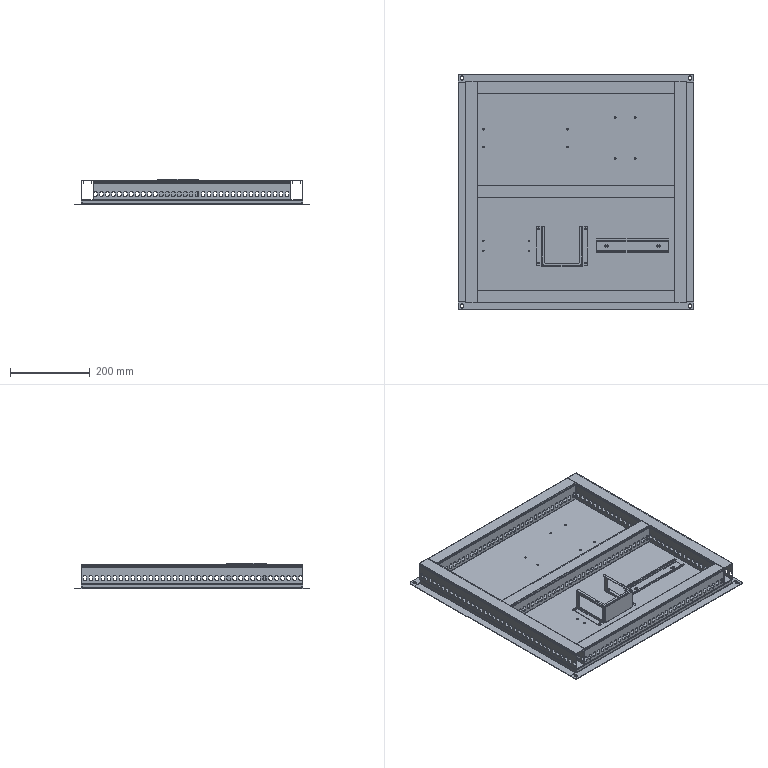Part | SolidWorks | 8 solids | 1940 faces | box 590 x 590 x 63.5 mm | volume 996425 mm3 | plane 1098 | cylinder 830 | spline 12 | commonest cylinder face diameters 8 x692 4 x40 3 x36 1 x12 4.5 x8 7 x8